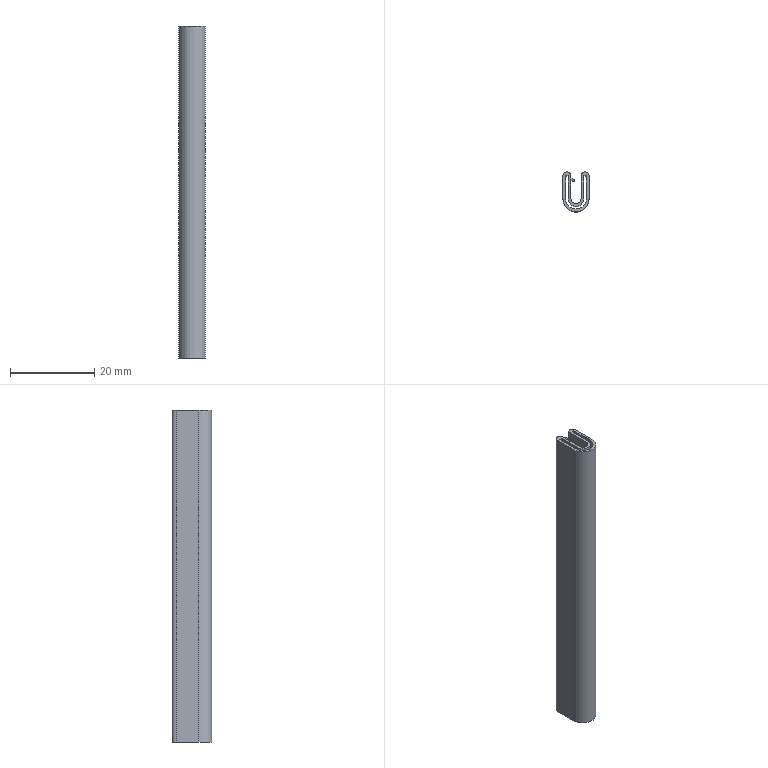Part | STEP file | TRAT2_4_B_3L2_TRAT2.4-B-3-L1 | 1 solid | 22 faces | box 6.2 x 9.5 x 79 mm | volume 2037 mm3 | plane 15 | cylinder 7 | commonest cylinder face diameters 1.9 x2 0.4 x1 2.4 x1 3.692 x1 4.933 x1 6.2 x1
STEP:
#1=CARTESIAN_POINT('',(1.9,8.55,79.));
#2=VERTEX_POINT('',#1);
#3=CARTESIAN_POINT('',(0.,8.55,79.));
#4=VERTEX_POINT('',#3);
#5=CARTESIAN_POINT('',(0.95,8.55,79.));
#6=DIRECTION('',(0.,0.,1.));
#7=DIRECTION('',(1.,0.,0.));
#8=AXIS2_PLACEMENT_3D('',#5,#6,#7);
#9=CIRCLE('',#8,0.95);
#10=EDGE_CURVE('',#2,#4,#9,.T.);
#11=ORIENTED_EDGE('',*,*,#10,.T.);
#12=CARTESIAN_POINT('',(0.,3.1,79.));
#13=VERTEX_POINT('',#12);
#14=CARTESIAN_POINT('',(0.,8.55,79.));
#15=DIRECTION('',(0.,-1.,0.));
#16=VECTOR('',#15,1000.);
#17=LINE('',#14,#16);
#18=EDGE_CURVE('',#4,#13,#17,.T.);
#19=ORIENTED_EDGE('',*,*,#18,.T.);
#20=CARTESIAN_POINT('',(6.2,3.1,79.));
#21=VERTEX_POINT('',#20);
#22=CARTESIAN_POINT('',(3.1,3.1,79.));
#23=DIRECTION('',(0.,0.,1.));
#24=DIRECTION('',(1.,0.,0.));
#25=AXIS2_PLACEMENT_3D('',#22,#23,#24);
#26=CIRCLE('',#25,3.1);
#27=EDGE_CURVE('',#13,#21,#26,.T.);
#28=ORIENTED_EDGE('',*,*,#27,.T.);
#29=CARTESIAN_POINT('',(6.2,8.55,79.));
#30=VERTEX_POINT('',#29);
#31=CARTESIAN_POINT('',(6.2,3.1,79.));
#32=DIRECTION('',(0.,1.,0.));
#33=VECTOR('',#32,1000.);
#34=LINE('',#31,#33);
#35=EDGE_CURVE('',#21,#30,#34,.T.);
#36=ORIENTED_EDGE('',*,*,#35,.T.);
#37=CARTESIAN_POINT('',(4.3,8.55,79.));
#38=VERTEX_POINT('',#37);
#39=CARTESIAN_POINT('',(5.25,8.55,79.));
#40=DIRECTION('',(0.,0.,1.));
#41=DIRECTION('',(1.,0.,0.));
#42=AXIS2_PLACEMENT_3D('',#39,#40,#41);
#43=CIRCLE('',#42,0.95);
#44=EDGE_CURVE('',#30,#38,#43,.T.);
#45=ORIENTED_EDGE('',*,*,#44,.T.);
#46=CARTESIAN_POINT('',(4.3,3.1,79.));
#47=VERTEX_POINT('',#46);
#48=CARTESIAN_POINT('',(4.3,8.55,79.));
#49=DIRECTION('',(0.,-1.,0.));
#50=VECTOR('',#49,1000.);
#51=LINE('',#48,#50);
#52=EDGE_CURVE('',#38,#47,#51,.T.);
#53=ORIENTED_EDGE('',*,*,#52,.T.);
#54=CARTESIAN_POINT('',(1.9,3.1,79.));
#55=VERTEX_POINT('',#54);
#56=CARTESIAN_POINT('',(3.1,3.1,79.));
#57=DIRECTION('',(0.,0.,-1.));
#58=DIRECTION('',(-1.,0.,0.));
#59=AXIS2_PLACEMENT_3D('',#56,#57,#58);
#60=CIRCLE('',#59,1.2);
#61=EDGE_CURVE('',#47,#55,#60,.T.);
#62=ORIENTED_EDGE('',*,*,#61,.T.);
#63=CARTESIAN_POINT('',(1.9,7.6,79.));
#64=VERTEX_POINT('',#63);
#65=CARTESIAN_POINT('',(1.9,3.1,79.));
#66=DIRECTION('',(0.,1.,0.));
#67=VECTOR('',#66,1000.);
#68=LINE('',#65,#67);
#69=EDGE_CURVE('',#55,#64,#68,.T.);
#70=ORIENTED_EDGE('',*,*,#69,.T.);
#71=CARTESIAN_POINT('',(2.472,7.27,79.));
#72=VERTEX_POINT('',#71);
#73=CARTESIAN_POINT('',(1.9,7.6,79.));
#74=DIRECTION('',(0.866,-0.5,0.));
#75=VECTOR('',#74,1000.);
#76=LINE('',#73,#75);
#77=EDGE_CURVE('',#64,#72,#76,.T.);
#78=ORIENTED_EDGE('',*,*,#77,.T.);
#79=CARTESIAN_POINT('',(2.672,7.616,79.));
#80=VERTEX_POINT('',#79);
#81=CARTESIAN_POINT('',(2.572,7.443,79.));
#82=DIRECTION('',(0.,0.,1.));
#83=DIRECTION('',(1.,0.,0.));
#84=AXIS2_PLACEMENT_3D('',#81,#82,#83);
#85=CIRCLE('',#84,0.2);
#86=EDGE_CURVE('',#72,#80,#85,.T.);
#87=ORIENTED_EDGE('',*,*,#86,.T.);
#88=CARTESIAN_POINT('',(1.9,8.062,79.));
#89=VERTEX_POINT('',#88);
#90=CARTESIAN_POINT('',(2.672,7.616,79.));
#91=DIRECTION('',(-0.866,0.5,0.));
#92=VECTOR('',#91,1000.);
#93=LINE('',#90,#92);
#94=EDGE_CURVE('',#80,#89,#93,.T.);
#95=ORIENTED_EDGE('',*,*,#94,.T.);
#96=CARTESIAN_POINT('',(1.9,8.062,79.));
#97=DIRECTION('',(0.,1.,0.));
#98=VECTOR('',#97,1000.);
#99=LINE('',#96,#98);
#100=EDGE_CURVE('',#89,#2,#99,.T.);
#101=ORIENTED_EDGE('',*,*,#100,.T.);
#102=EDGE_LOOP('',(#11,#19,#28,#36,#45,#53,#62,#70,#78,#87,#95,#101));
#103=FACE_OUTER_BOUND('',#102,.T.);
#104=CARTESIAN_POINT('',(0.6333,8.55,79.));
#105=VERTEX_POINT('',#104);
#106=CARTESIAN_POINT('',(0.6333,3.1,79.));
#107=VERTEX_POINT('',#106);
#108=CARTESIAN_POINT('',(0.6333,8.55,79.));
#109=DIRECTION('',(0.,-1.,0.));
#110=VECTOR('',#109,1000.);
#111=LINE('',#108,#110);
#112=EDGE_CURVE('',#105,#107,#111,.T.);
#113=ORIENTED_EDGE('',*,*,#112,.F.);
#114=CARTESIAN_POINT('',(1.254,8.55,79.));
#115=VERTEX_POINT('',#114);
#116=CARTESIAN_POINT('',(1.254,8.55,79.));
#117=DIRECTION('',(-1.,0.,0.));
#118=VECTOR('',#117,1000.);
#119=LINE('',#116,#118);
#120=EDGE_CURVE('',#115,#105,#119,.T.);
#121=ORIENTED_EDGE('',*,*,#120,.F.);
#122=CARTESIAN_POINT('',(1.254,3.1,79.));
#123=VERTEX_POINT('',#122);
#124=CARTESIAN_POINT('',(1.254,3.1,79.));
#125=DIRECTION('',(0.,1.,0.));
#126=VECTOR('',#125,1000.);
#127=LINE('',#124,#126);
#128=EDGE_CURVE('',#123,#115,#127,.T.);
#129=ORIENTED_EDGE('',*,*,#128,.F.);
#130=CARTESIAN_POINT('',(4.946,3.1,79.));
#131=VERTEX_POINT('',#130);
#132=CARTESIAN_POINT('',(3.1,3.1,79.));
#133=DIRECTION('',(0.,0.,-1.));
#134=DIRECTION('',(-1.,0.,0.));
#135=AXIS2_PLACEMENT_3D('',#132,#133,#134);
#136=CIRCLE('',#135,1.846);
#137=EDGE_CURVE('',#131,#123,#136,.T.);
#138=ORIENTED_EDGE('',*,*,#137,.F.);
#139=CARTESIAN_POINT('',(4.946,8.55,79.));
#140=VERTEX_POINT('',#139);
#141=CARTESIAN_POINT('',(4.946,8.55,79.));
#142=DIRECTION('',(0.,-1.,0.));
#143=VECTOR('',#142,1000.);
#144=LINE('',#141,#143);
#145=EDGE_CURVE('',#140,#131,#144,.T.);
#146=ORIENTED_EDGE('',*,*,#145,.F.);
#147=CARTESIAN_POINT('',(5.567,8.55,79.));
#148=VERTEX_POINT('',#147);
#149=CARTESIAN_POINT('',(5.567,8.55,79.));
#150=DIRECTION('',(-1.,0.,0.));
#151=VECTOR('',#150,1000.);
#152=LINE('',#149,#151);
#153=EDGE_CURVE('',#148,#140,#152,.T.);
#154=ORIENTED_EDGE('',*,*,#153,.F.);
#155=CARTESIAN_POINT('',(5.567,3.1,79.));
#156=VERTEX_POINT('',#155);
#157=CARTESIAN_POINT('',(5.567,3.1,79.));
#158=DIRECTION('',(0.,1.,0.));
#159=VECTOR('',#158,1000.);
#160=LINE('',#157,#159);
#161=EDGE_CURVE('',#156,#148,#160,.T.);
#162=ORIENTED_EDGE('',*,*,#161,.F.);
#163=CARTESIAN_POINT('',(3.1,3.1,79.));
#164=DIRECTION('',(0.,0.,1.));
#165=DIRECTION('',(1.,0.,0.));
#166=AXIS2_PLACEMENT_3D('',#163,#164,#165);
#167=CIRCLE('',#166,2.467);
#168=EDGE_CURVE('',#107,#156,#167,.T.);
#169=ORIENTED_EDGE('',*,*,#168,.F.);
#170=EDGE_LOOP('',(#113,#121,#129,#138,#146,#154,#162,#169));
#171=FACE_BOUND('',#170,.T.);
#172=CARTESIAN_POINT('',(0.95,8.55,79.));
#173=DIRECTION('',(0.,0.,1.));
#174=DIRECTION('',(1.,0.,0.));
#175=AXIS2_PLACEMENT_3D('',#172,#173,#174);
#176=PLANE('',#175);
#177=ADVANCED_FACE('',(#103,#171),#176,.T.);
#178=CARTESIAN_POINT('',(1.9,8.55,0.));
#179=VERTEX_POINT('',#178);
#180=CARTESIAN_POINT('',(0.,8.55,0.));
#181=VERTEX_POINT('',#180);
#182=CARTESIAN_POINT('',(0.95,8.55,0.));
#183=DIRECTION('',(0.,0.,1.));
#184=DIRECTION('',(1.,0.,0.));
#185=AXIS2_PLACEMENT_3D('',#182,#183,#184);
#186=CIRCLE('',#185,0.95);
#187=EDGE_CURVE('',#179,#181,#186,.T.);
#188=ORIENTED_EDGE('',*,*,#187,.F.);
#189=CARTESIAN_POINT('',(1.9,8.062,0.));
#190=VERTEX_POINT('',#189);
#191=CARTESIAN_POINT('',(1.9,8.062,0.));
#192=DIRECTION('',(0.,1.,0.));
#193=VECTOR('',#192,1000.);
#194=LINE('',#191,#193);
#195=EDGE_CURVE('',#190,#179,#194,.T.);
#196=ORIENTED_EDGE('',*,*,#195,.F.);
#197=CARTESIAN_POINT('',(2.672,7.616,0.));
#198=VERTEX_POINT('',#197);
#199=CARTESIAN_POINT('',(2.672,7.616,0.));
#200=DIRECTION('',(-0.866,0.5,0.));
#201=VECTOR('',#200,1000.);
#202=LINE('',#199,#201);
#203=EDGE_CURVE('',#198,#190,#202,.T.);
#204=ORIENTED_EDGE('',*,*,#203,.F.);
#205=CARTESIAN_POINT('',(2.472,7.27,0.));
#206=VERTEX_POINT('',#205);
#207=CARTESIAN_POINT('',(2.572,7.443,0.));
#208=DIRECTION('',(0.,0.,1.));
#209=DIRECTION('',(1.,0.,0.));
#210=AXIS2_PLACEMENT_3D('',#207,#208,#209);
#211=CIRCLE('',#210,0.2);
#212=EDGE_CURVE('',#206,#198,#211,.T.);
#213=ORIENTED_EDGE('',*,*,#212,.F.);
#214=CARTESIAN_POINT('',(1.9,7.6,0.));
#215=VERTEX_POINT('',#214);
#216=CARTESIAN_POINT('',(1.9,7.6,0.));
#217=DIRECTION('',(0.866,-0.5,0.));
#218=VECTOR('',#217,1000.);
#219=LINE('',#216,#218);
#220=EDGE_CURVE('',#215,#206,#219,.T.);
#221=ORIENTED_EDGE('',*,*,#220,.F.);
#222=CARTESIAN_POINT('',(1.9,3.1,0.));
#223=VERTEX_POINT('',#222);
#224=CARTESIAN_POINT('',(1.9,3.1,0.));
#225=DIRECTION('',(0.,1.,0.));
#226=VECTOR('',#225,1000.);
#227=LINE('',#224,#226);
#228=EDGE_CURVE('',#223,#215,#227,.T.);
#229=ORIENTED_EDGE('',*,*,#228,.F.);
#230=CARTESIAN_POINT('',(4.3,3.1,0.));
#231=VERTEX_POINT('',#230);
#232=CARTESIAN_POINT('',(3.1,3.1,0.));
#233=DIRECTION('',(0.,0.,-1.));
#234=DIRECTION('',(-1.,0.,0.));
#235=AXIS2_PLACEMENT_3D('',#232,#233,#234);
#236=CIRCLE('',#235,1.2);
#237=EDGE_CURVE('',#231,#223,#236,.T.);
#238=ORIENTED_EDGE('',*,*,#237,.F.);
#239=CARTESIAN_POINT('',(4.3,8.55,0.));
#240=VERTEX_POINT('',#239);
#241=CARTESIAN_POINT('',(4.3,8.55,0.));
#242=DIRECTION('',(0.,-1.,0.));
#243=VECTOR('',#242,1000.);
#244=LINE('',#241,#243);
#245=EDGE_CURVE('',#240,#231,#244,.T.);
#246=ORIENTED_EDGE('',*,*,#245,.F.);
#247=CARTESIAN_POINT('',(6.2,8.55,0.));
#248=VERTEX_POINT('',#247);
#249=CARTESIAN_POINT('',(5.25,8.55,0.));
#250=DIRECTION('',(0.,0.,1.));
#251=DIRECTION('',(1.,0.,0.));
#252=AXIS2_PLACEMENT_3D('',#249,#250,#251);
#253=CIRCLE('',#252,0.95);
#254=EDGE_CURVE('',#248,#240,#253,.T.);
#255=ORIENTED_EDGE('',*,*,#254,.F.);
#256=CARTESIAN_POINT('',(6.2,3.1,0.));
#257=VERTEX_POINT('',#256);
#258=CARTESIAN_POINT('',(6.2,3.1,0.));
#259=DIRECTION('',(0.,1.,0.));
#260=VECTOR('',#259,1000.);
#261=LINE('',#258,#260);
#262=EDGE_CURVE('',#257,#248,#261,.T.);
#263=ORIENTED_EDGE('',*,*,#262,.F.);
#264=CARTESIAN_POINT('',(0.,3.1,0.));
#265=VERTEX_POINT('',#264);
#266=CARTESIAN_POINT('',(3.1,3.1,0.));
#267=DIRECTION('',(0.,0.,1.));
#268=DIRECTION('',(1.,0.,0.));
#269=AXIS2_PLACEMENT_3D('',#266,#267,#268);
#270=CIRCLE('',#269,3.1);
#271=EDGE_CURVE('',#265,#257,#270,.T.);
#272=ORIENTED_EDGE('',*,*,#271,.F.);
#273=CARTESIAN_POINT('',(0.,8.55,0.));
#274=DIRECTION('',(0.,-1.,0.));
#275=VECTOR('',#274,1000.);
#276=LINE('',#273,#275);
#277=EDGE_CURVE('',#181,#265,#276,.T.);
#278=ORIENTED_EDGE('',*,*,#277,.F.);
#279=EDGE_LOOP('',(#188,#196,#204,#213,#221,#229,#238,#246,#255,#263,#272,#278));
#280=FACE_OUTER_BOUND('',#279,.T.);
#281=CARTESIAN_POINT('',(1.254,8.55,0.));
#282=VERTEX_POINT('',#281);
#283=CARTESIAN_POINT('',(0.6333,8.55,0.));
#284=VERTEX_POINT('',#283);
#285=CARTESIAN_POINT('',(1.254,8.55,0.));
#286=DIRECTION('',(-1.,0.,0.));
#287=VECTOR('',#286,1000.);
#288=LINE('',#285,#287);
#289=EDGE_CURVE('',#282,#284,#288,.T.);
#290=ORIENTED_EDGE('',*,*,#289,.T.);
#291=CARTESIAN_POINT('',(0.6333,3.1,0.));
#292=VERTEX_POINT('',#291);
#293=CARTESIAN_POINT('',(0.6333,8.55,0.));
#294=DIRECTION('',(0.,-1.,0.));
#295=VECTOR('',#294,1000.);
#296=LINE('',#293,#295);
#297=EDGE_CURVE('',#284,#292,#296,.T.);
#298=ORIENTED_EDGE('',*,*,#297,.T.);
#299=CARTESIAN_POINT('',(5.567,3.1,0.));
#300=VERTEX_POINT('',#299);
#301=CARTESIAN_POINT('',(3.1,3.1,0.));
#302=DIRECTION('',(0.,0.,1.));
#303=DIRECTION('',(1.,0.,0.));
#304=AXIS2_PLACEMENT_3D('',#301,#302,#303);
#305=CIRCLE('',#304,2.467);
#306=EDGE_CURVE('',#292,#300,#305,.T.);
#307=ORIENTED_EDGE('',*,*,#306,.T.);
#308=CARTESIAN_POINT('',(5.567,8.55,0.));
#309=VERTEX_POINT('',#308);
#310=CARTESIAN_POINT('',(5.567,3.1,0.));
#311=DIRECTION('',(0.,1.,0.));
#312=VECTOR('',#311,1000.);
#313=LINE('',#310,#312);
#314=EDGE_CURVE('',#300,#309,#313,.T.);
#315=ORIENTED_EDGE('',*,*,#314,.T.);
#316=CARTESIAN_POINT('',(4.946,8.55,0.));
#317=VERTEX_POINT('',#316);
#318=CARTESIAN_POINT('',(5.567,8.55,0.));
#319=DIRECTION('',(-1.,0.,0.));
#320=VECTOR('',#319,1000.);
#321=LINE('',#318,#320);
#322=EDGE_CURVE('',#309,#317,#321,.T.);
#323=ORIENTED_EDGE('',*,*,#322,.T.);
#324=CARTESIAN_POINT('',(4.946,3.1,0.));
#325=VERTEX_POINT('',#324);
#326=CARTESIAN_POINT('',(4.946,8.55,0.));
#327=DIRECTION('',(0.,-1.,0.));
#328=VECTOR('',#327,1000.);
#329=LINE('',#326,#328);
#330=EDGE_CURVE('',#317,#325,#329,.T.);
#331=ORIENTED_EDGE('',*,*,#330,.T.);
#332=CARTESIAN_POINT('',(1.254,3.1,0.));
#333=VERTEX_POINT('',#332);
#334=CARTESIAN_POINT('',(3.1,3.1,0.));
#335=DIRECTION('',(0.,0.,-1.));
#336=DIRECTION('',(-1.,0.,0.));
#337=AXIS2_PLACEMENT_3D('',#334,#335,#336);
#338=CIRCLE('',#337,1.846);
#339=EDGE_CURVE('',#325,#333,#338,.T.);
#340=ORIENTED_EDGE('',*,*,#339,.T.);
#341=CARTESIAN_POINT('',(1.254,3.1,0.));
#342=DIRECTION('',(0.,1.,0.));
#343=VECTOR('',#342,1000.);
#344=LINE('',#341,#343);
#345=EDGE_CURVE('',#333,#282,#344,.T.);
#346=ORIENTED_EDGE('',*,*,#345,.T.);
#347=EDGE_LOOP('',(#290,#298,#307,#315,#323,#331,#340,#346));
#348=FACE_BOUND('',#347,.T.);
#349=CARTESIAN_POINT('',(0.95,8.55,0.));
#350=DIRECTION('',(0.,0.,1.));
#351=DIRECTION('',(1.,0.,0.));
#352=AXIS2_PLACEMENT_3D('',#349,#350,#351);
#353=PLANE('',#352);
#354=ADVANCED_FACE('',(#280,#348),#353,.F.);
#355=ORIENTED_EDGE('',*,*,#187,.T.);
#356=CARTESIAN_POINT('',(0.,8.55,79.));
#357=DIRECTION('',(0.,0.,-1.));
#358=VECTOR('',#357,1000.);
#359=LINE('',#356,#358);
#360=EDGE_CURVE('',#4,#181,#359,.T.);
#361=ORIENTED_EDGE('',*,*,#360,.F.);
#362=ORIENTED_EDGE('',*,*,#10,.F.);
#363=CARTESIAN_POINT('',(1.9,8.55,79.));
#364=DIRECTION('',(0.,0.,-1.));
#365=VECTOR('',#364,1000.);
#366=LINE('',#363,#365);
#367=EDGE_CURVE('',#2,#179,#366,.T.);
#368=ORIENTED_EDGE('',*,*,#367,.T.);
#369=EDGE_LOOP('',(#355,#361,#362,#368));
#370=FACE_OUTER_BOUND('',#369,.T.);
#371=CARTESIAN_POINT('',(0.95,8.55,79.));
#372=DIRECTION('',(0.,0.,-1.));
#373=DIRECTION('',(-1.,0.,0.));
#374=AXIS2_PLACEMENT_3D('',#371,#372,#373);
#375=CYLINDRICAL_SURFACE('',#374,0.95);
#376=ADVANCED_FACE('',(#370),#375,.T.);
#377=ORIENTED_EDGE('',*,*,#277,.T.);
#378=CARTESIAN_POINT('',(0.,3.1,79.));
#379=DIRECTION('',(0.,0.,-1.));
#380=VECTOR('',#379,1000.);
#381=LINE('',#378,#380);
#382=EDGE_CURVE('',#13,#265,#381,.T.);
#383=ORIENTED_EDGE('',*,*,#382,.F.);
#384=ORIENTED_EDGE('',*,*,#18,.F.);
#385=ORIENTED_EDGE('',*,*,#360,.T.);
#386=EDGE_LOOP('',(#377,#383,#384,#385));
#387=FACE_OUTER_BOUND('',#386,.T.);
#388=CARTESIAN_POINT('',(0.,8.55,79.));
#389=DIRECTION('',(1.,0.,0.));
#390=DIRECTION('',(0.,0.,-1.));
#391=AXIS2_PLACEMENT_3D('',#388,#389,#390);
#392=PLANE('',#391);
#393=ADVANCED_FACE('',(#387),#392,.F.);
#394=ORIENTED_EDGE('',*,*,#271,.T.);
#395=CARTESIAN_POINT('',(6.2,3.1,79.));
#396=DIRECTION('',(0.,0.,-1.));
#397=VECTOR('',#396,1000.);
#398=LINE('',#395,#397);
#399=EDGE_CURVE('',#21,#257,#398,.T.);
#400=ORIENTED_EDGE('',*,*,#399,.F.);
#401=ORIENTED_EDGE('',*,*,#27,.F.);
#402=ORIENTED_EDGE('',*,*,#382,.T.);
#403=EDGE_LOOP('',(#394,#400,#401,#402));
#404=FACE_OUTER_BOUND('',#403,.T.);
#405=CARTESIAN_POINT('',(3.1,3.1,79.));
#406=DIRECTION('',(0.,0.,-1.));
#407=DIRECTION('',(-1.,0.,0.));
#408=AXIS2_PLACEMENT_3D('',#405,#406,#407);
#409=CYLINDRICAL_SURFACE('',#408,3.1);
#410=ADVANCED_FACE('',(#404),#409,.T.);
#411=ORIENTED_EDGE('',*,*,#262,.T.);
#412=CARTESIAN_POINT('',(6.2,8.55,79.));
#413=DIRECTION('',(0.,0.,-1.));
#414=VECTOR('',#413,1000.);
#415=LINE('',#412,#414);
#416=EDGE_CURVE('',#30,#248,#415,.T.);
#417=ORIENTED_EDGE('',*,*,#416,.F.);
#418=ORIENTED_EDGE('',*,*,#35,.F.);
#419=ORIENTED_EDGE('',*,*,#399,.T.);
#420=EDGE_LOOP('',(#411,#417,#418,#419));
#421=FACE_OUTER_BOUND('',#420,.T.);
#422=CARTESIAN_POINT('',(6.2,3.1,79.));
#423=DIRECTION('',(-1.,0.,0.));
#424=DIRECTION('',(0.,0.,1.));
#425=AXIS2_PLACEMENT_3D('',#422,#423,#424);
#426=PLANE('',#425);
#427=ADVANCED_FACE('',(#421),#426,.F.);
#428=ORIENTED_EDGE('',*,*,#254,.T.);
#429=CARTESIAN_POINT('',(4.3,8.55,79.));
#430=DIRECTION('',(0.,0.,-1.));
#431=VECTOR('',#430,1000.);
#432=LINE('',#429,#431);
#433=EDGE_CURVE('',#38,#240,#432,.T.);
#434=ORIENTED_EDGE('',*,*,#433,.F.);
#435=ORIENTED_EDGE('',*,*,#44,.F.);
#436=ORIENTED_EDGE('',*,*,#416,.T.);
#437=EDGE_LOOP('',(#428,#434,#435,#436));
#438=FACE_OUTER_BOUND('',#437,.T.);
#439=CARTESIAN_POINT('',(5.25,8.55,79.));
#440=DIRECTION('',(0.,0.,-1.));
#441=DIRECTION('',(-1.,0.,0.));
#442=AXIS2_PLACEMENT_3D('',#439,#440,#441);
#443=CYLINDRICAL_SURFACE('',#442,0.95);
#444=ADVANCED_FACE('',(#438),#443,.T.);
#445=ORIENTED_EDGE('',*,*,#245,.T.);
#446=CARTESIAN_POINT('',(4.3,3.1,79.));
#447=DIRECTION('',(0.,0.,-1.));
#448=VECTOR('',#447,1000.);
#449=LINE('',#446,#448);
#450=EDGE_CURVE('',#47,#231,#449,.T.);
#451=ORIENTED_EDGE('',*,*,#450,.F.);
#452=ORIENTED_EDGE('',*,*,#52,.F.);
#453=ORIENTED_EDGE('',*,*,#433,.T.);
#454=EDGE_LOOP('',(#445,#451,#452,#453));
#455=FACE_OUTER_BOUND('',#454,.T.);
#456=CARTESIAN_POINT('',(4.3,8.55,79.));
#457=DIRECTION('',(1.,0.,0.));
#458=DIRECTION('',(0.,1.,0.));
#459=AXIS2_PLACEMENT_3D('',#456,#457,#458);
#460=PLANE('',#459);
#461=ADVANCED_FACE('',(#455),#460,.F.);
#462=ORIENTED_EDGE('',*,*,#237,.T.);
#463=CARTESIAN_POINT('',(1.9,3.1,79.));
#464=DIRECTION('',(0.,0.,-1.));
#465=VECTOR('',#464,1000.);
#466=LINE('',#463,#465);
#467=EDGE_CURVE('',#55,#223,#466,.T.);
#468=ORIENTED_EDGE('',*,*,#467,.F.);
#469=ORIENTED_EDGE('',*,*,#61,.F.);
#470=ORIENTED_EDGE('',*,*,#450,.T.);
#471=EDGE_LOOP('',(#462,#468,#469,#470));
#472=FACE_OUTER_BOUND('',#471,.T.);
#473=CARTESIAN_POINT('',(3.1,3.1,79.));
#474=DIRECTION('',(0.,0.,-1.));
#475=DIRECTION('',(-1.,0.,0.));
#476=AXIS2_PLACEMENT_3D('',#473,#474,#475);
#477=CYLINDRICAL_SURFACE('',#476,1.2);
#478=ADVANCED_FACE('',(#472),#477,.F.);
#479=ORIENTED_EDGE('',*,*,#228,.T.);
#480=CARTESIAN_POINT('',(1.9,7.6,79.));
#481=DIRECTION('',(0.,0.,-1.));
#482=VECTOR('',#481,1000.);
#483=LINE('',#480,#482);
#484=EDGE_CURVE('',#64,#215,#483,.T.);
#485=ORIENTED_EDGE('',*,*,#484,.F.);
#486=ORIENTED_EDGE('',*,*,#69,.F.);
#487=ORIENTED_EDGE('',*,*,#467,.T.);
#488=EDGE_LOOP('',(#479,#485,#486,#487));
#489=FACE_OUTER_BOUND('',#488,.T.);
#490=CARTESIAN_POINT('',(1.9,3.1,79.));
#491=DIRECTION('',(-1.,0.,0.));
#492=DIRECTION('',(0.,-1.,0.));
#493=AXIS2_PLACEMENT_3D('',#490,#491,#492);
#494=PLANE('',#493);
#495=ADVANCED_FACE('',(#489),#494,.F.);
#496=ORIENTED_EDGE('',*,*,#220,.T.);
#497=CARTESIAN_POINT('',(2.472,7.27,79.));
#498=DIRECTION('',(0.,0.,-1.));
#499=VECTOR('',#498,1000.);
#500=LINE('',#497,#499);
#501=EDGE_CURVE('',#72,#206,#500,.T.);
#502=ORIENTED_EDGE('',*,*,#501,.F.);
#503=ORIENTED_EDGE('',*,*,#77,.F.);
#504=ORIENTED_EDGE('',*,*,#484,.T.);
#505=EDGE_LOOP('',(#496,#502,#503,#504));
#506=FACE_OUTER_BOUND('',#505,.T.);
#507=CARTESIAN_POINT('',(1.9,7.6,79.));
#508=DIRECTION('',(0.5,0.866,0.));
#509=DIRECTION('',(-0.866,0.5,0.));
#510=AXIS2_PLACEMENT_3D('',#507,#508,#509);
#511=PLANE('',#510);
#512=ADVANCED_FACE('',(#506),#511,.F.);
#513=ORIENTED_EDGE('',*,*,#212,.T.);
#514=CARTESIAN_POINT('',(2.672,7.616,79.));
#515=DIRECTION('',(0.,0.,-1.));
#516=VECTOR('',#515,1000.);
#517=LINE('',#514,#516);
#518=EDGE_CURVE('',#80,#198,#517,.T.);
#519=ORIENTED_EDGE('',*,*,#518,.F.);
#520=ORIENTED_EDGE('',*,*,#86,.F.);
#521=ORIENTED_EDGE('',*,*,#501,.T.);
#522=EDGE_LOOP('',(#513,#519,#520,#521));
#523=FACE_OUTER_BOUND('',#522,.T.);
#524=CARTESIAN_POINT('',(2.572,7.443,79.));
#525=DIRECTION('',(0.,0.,-1.));
#526=DIRECTION('',(-1.,0.,0.));
#527=AXIS2_PLACEMENT_3D('',#524,#525,#526);
#528=CYLINDRICAL_SURFACE('',#527,0.2);
#529=ADVANCED_FACE('',(#523),#528,.T.);
#530=ORIENTED_EDGE('',*,*,#203,.T.);
#531=CARTESIAN_POINT('',(1.9,8.062,79.));
#532=DIRECTION('',(0.,0.,-1.));
#533=VECTOR('',#532,1000.);
#534=LINE('',#531,#533);
#535=EDGE_CURVE('',#89,#190,#534,.T.);
#536=ORIENTED_EDGE('',*,*,#535,.F.);
#537=ORIENTED_EDGE('',*,*,#94,.F.);
#538=ORIENTED_EDGE('',*,*,#518,.T.);
#539=EDGE_LOOP('',(#530,#536,#537,#538));
#540=FACE_OUTER_BOUND('',#539,.T.);
#541=CARTESIAN_POINT('',(2.672,7.616,79.));
#542=DIRECTION('',(-0.5,-0.866,0.));
#543=DIRECTION('',(0.866,-0.5,0.));
#544=AXIS2_PLACEMENT_3D('',#541,#542,#543);
#545=PLANE('',#544);
#546=ADVANCED_FACE('',(#540),#545,.F.);
#547=ORIENTED_EDGE('',*,*,#195,.T.);
#548=ORIENTED_EDGE('',*,*,#367,.F.);
#549=ORIENTED_EDGE('',*,*,#100,.F.);
#550=ORIENTED_EDGE('',*,*,#535,.T.);
#551=EDGE_LOOP('',(#547,#548,#549,#550));
#552=FACE_OUTER_BOUND('',#551,.T.);
#553=CARTESIAN_POINT('',(1.9,8.062,79.));
#554=DIRECTION('',(-1.,0.,0.));
#555=DIRECTION('',(0.,0.,1.));
#556=AXIS2_PLACEMENT_3D('',#553,#554,#555);
#557=PLANE('',#556);
#558=ADVANCED_FACE('',(#552),#557,.F.);
#559=ORIENTED_EDGE('',*,*,#289,.F.);
#560=CARTESIAN_POINT('',(1.254,8.55,79.));
#561=DIRECTION('',(0.,0.,-1.));
#562=VECTOR('',#561,1000.);
#563=LINE('',#560,#562);
#564=EDGE_CURVE('',#115,#282,#563,.T.);
#565=ORIENTED_EDGE('',*,*,#564,.F.);
#566=ORIENTED_EDGE('',*,*,#120,.T.);
#567=CARTESIAN_POINT('',(0.6333,8.55,79.));
#568=DIRECTION('',(0.,0.,-1.));
#569=VECTOR('',#568,1000.);
#570=LINE('',#567,#569);
#571=EDGE_CURVE('',#105,#284,#570,.T.);
#572=ORIENTED_EDGE('',*,*,#571,.T.);
#573=EDGE_LOOP('',(#559,#565,#566,#572));
#574=FACE_OUTER_BOUND('',#573,.T.);
#575=CARTESIAN_POINT('',(1.254,8.55,79.));
#576=DIRECTION('',(0.,-1.,0.));
#577=DIRECTION('',(0.,0.,-1.));
#578=AXIS2_PLACEMENT_3D('',#575,#576,#577);
#579=PLANE('',#578);
#580=ADVANCED_FACE('',(#574),#579,.T.);
#581=ORIENTED_EDGE('',*,*,#297,.F.);
#582=ORIENTED_EDGE('',*,*,#571,.F.);
#583=ORIENTED_EDGE('',*,*,#112,.T.);
#584=CARTESIAN_POINT('',(0.6333,3.1,79.));
#585=DIRECTION('',(0.,0.,-1.));
#586=VECTOR('',#585,1000.);
#587=LINE('',#584,#586);
#588=EDGE_CURVE('',#107,#292,#587,.T.);
#589=ORIENTED_EDGE('',*,*,#588,.T.);
#590=EDGE_LOOP('',(#581,#582,#583,#589));
#591=FACE_OUTER_BOUND('',#590,.T.);
#592=CARTESIAN_POINT('',(0.6333,8.55,79.));
#593=DIRECTION('',(1.,0.,0.));
#594=DIRECTION('',(0.,1.,0.));
#595=AXIS2_PLACEMENT_3D('',#592,#593,#594);
#596=PLANE('',#595);
#597=ADVANCED_FACE('',(#591),#596,.T.);
#598=ORIENTED_EDGE('',*,*,#306,.F.);
#599=ORIENTED_EDGE('',*,*,#588,.F.);
#600=ORIENTED_EDGE('',*,*,#168,.T.);
#601=CARTESIAN_POINT('',(5.567,3.1,79.));
#602=DIRECTION('',(0.,0.,-1.));
#603=VECTOR('',#602,1000.);
#604=LINE('',#601,#603);
#605=EDGE_CURVE('',#156,#300,#604,.T.);
#606=ORIENTED_EDGE('',*,*,#605,.T.);
#607=EDGE_LOOP('',(#598,#599,#600,#606));
#608=FACE_OUTER_BOUND('',#607,.T.);
#609=CARTESIAN_POINT('',(3.1,3.1,79.));
#610=DIRECTION('',(0.,0.,-1.));
#611=DIRECTION('',(-1.,0.,0.));
#612=AXIS2_PLACEMENT_3D('',#609,#610,#611);
#613=CYLINDRICAL_SURFACE('',#612,2.467);
#614=ADVANCED_FACE('',(#608),#613,.F.);
#615=ORIENTED_EDGE('',*,*,#314,.F.);
#616=ORIENTED_EDGE('',*,*,#605,.F.);
#617=ORIENTED_EDGE('',*,*,#161,.T.);
#618=CARTESIAN_POINT('',(5.567,8.55,79.));
#619=DIRECTION('',(0.,0.,-1.));
#620=VECTOR('',#619,1000.);
#621=LINE('',#618,#620);
#622=EDGE_CURVE('',#148,#309,#621,.T.);
#623=ORIENTED_EDGE('',*,*,#622,.T.);
#624=EDGE_LOOP('',(#615,#616,#617,#623));
#625=FACE_OUTER_BOUND('',#624,.T.);
#626=CARTESIAN_POINT('',(5.567,3.1,79.));
#627=DIRECTION('',(-1.,0.,0.));
#628=DIRECTION('',(0.,-1.,0.));
#629=AXIS2_PLACEMENT_3D('',#626,#627,#628);
#630=PLANE('',#629);
#631=ADVANCED_FACE('',(#625),#630,.T.);
#632=ORIENTED_EDGE('',*,*,#322,.F.);
#633=ORIENTED_EDGE('',*,*,#622,.F.);
#634=ORIENTED_EDGE('',*,*,#153,.T.);
#635=CARTESIAN_POINT('',(4.946,8.55,79.));
#636=DIRECTION('',(0.,0.,-1.));
#637=VECTOR('',#636,1000.);
#638=LINE('',#635,#637);
#639=EDGE_CURVE('',#140,#317,#638,.T.);
#640=ORIENTED_EDGE('',*,*,#639,.T.);
#641=EDGE_LOOP('',(#632,#633,#634,#640));
#642=FACE_OUTER_BOUND('',#641,.T.);
#643=CARTESIAN_POINT('',(5.567,8.55,79.));
#644=DIRECTION('',(0.,-1.,0.));
#645=DIRECTION('',(0.,0.,-1.));
#646=AXIS2_PLACEMENT_3D('',#643,#644,#645);
#647=PLANE('',#646);
#648=ADVANCED_FACE('',(#642),#647,.T.);
#649=ORIENTED_EDGE('',*,*,#330,.F.);
#650=ORIENTED_EDGE('',*,*,#639,.F.);
#651=ORIENTED_EDGE('',*,*,#145,.T.);
#652=CARTESIAN_POINT('',(4.946,3.1,79.));
#653=DIRECTION('',(0.,0.,-1.));
#654=VECTOR('',#653,1000.);
#655=LINE('',#652,#654);
#656=EDGE_CURVE('',#131,#325,#655,.T.);
#657=ORIENTED_EDGE('',*,*,#656,.T.);
#658=EDGE_LOOP('',(#649,#650,#651,#657));
#659=FACE_OUTER_BOUND('',#658,.T.);
#660=CARTESIAN_POINT('',(4.946,8.55,79.));
#661=DIRECTION('',(1.,0.,0.));
#662=DIRECTION('',(0.,0.,-1.));
#663=AXIS2_PLACEMENT_3D('',#660,#661,#662);
#664=PLANE('',#663);
#665=ADVANCED_FACE('',(#659),#664,.T.);
#666=ORIENTED_EDGE('',*,*,#339,.F.);
#667=ORIENTED_EDGE('',*,*,#656,.F.);
#668=ORIENTED_EDGE('',*,*,#137,.T.);
#669=CARTESIAN_POINT('',(1.254,3.1,79.));
#670=DIRECTION('',(0.,0.,-1.));
#671=VECTOR('',#670,1000.);
#672=LINE('',#669,#671);
#673=EDGE_CURVE('',#123,#333,#672,.T.);
#674=ORIENTED_EDGE('',*,*,#673,.T.);
#675=EDGE_LOOP('',(#666,#667,#668,#674));
#676=FACE_OUTER_BOUND('',#675,.T.);
#677=CARTESIAN_POINT('',(3.1,3.1,79.));
#678=DIRECTION('',(0.,0.,-1.));
#679=DIRECTION('',(-1.,0.,0.));
#680=AXIS2_PLACEMENT_3D('',#677,#678,#679);
#681=CYLINDRICAL_SURFACE('',#680,1.846);
#682=ADVANCED_FACE('',(#676),#681,.T.);
#683=ORIENTED_EDGE('',*,*,#345,.F.);
#684=ORIENTED_EDGE('',*,*,#673,.F.);
#685=ORIENTED_EDGE('',*,*,#128,.T.);
#686=ORIENTED_EDGE('',*,*,#564,.T.);
#687=EDGE_LOOP('',(#683,#684,#685,#686));
#688=FACE_OUTER_BOUND('',#687,.T.);
#689=CARTESIAN_POINT('',(1.254,3.1,79.));
#690=DIRECTION('',(-1.,0.,0.));
#691=DIRECTION('',(0.,-1.,0.));
#692=AXIS2_PLACEMENT_3D('',#689,#690,#691);
#693=PLANE('',#692);
#694=ADVANCED_FACE('',(#688),#693,.T.);
#695=CLOSED_SHELL('',(#177,#354,#376,#393,#410,#427,#444,#461,#478,#495,#512,#529,#546,#558,#580,#597,#614,#631,#648,#665,#682,#694));
#696=MANIFOLD_SOLID_BREP('',#695);
#697=CARTESIAN_POINT('',(0.,0.,0.));
#698=DIRECTION('',(0.,0.,1.));
#699=DIRECTION('',(1.,0.,0.));
#700=AXIS2_PLACEMENT_3D('',#697,#698,#699);
#701=(LENGTH_UNIT()NAMED_UNIT(*)SI_UNIT(.MILLI.,.METRE.));
#702=UNCERTAINTY_MEASURE_WITH_UNIT(LENGTH_MEASURE(0.00001),#701,'','');
#703=(NAMED_UNIT(*)PLANE_ANGLE_UNIT()SI_UNIT($,.RADIAN.));
#704=(NAMED_UNIT(*)SI_UNIT($,.STERADIAN.)SOLID_ANGLE_UNIT());
#705=(GEOMETRIC_REPRESENTATION_CONTEXT(3)GLOBAL_UNCERTAINTY_ASSIGNED_CONTEXT((#702))GLOBAL_UNIT_ASSIGNED_CONTEXT((#701,#703,#704))REPRESENTATION_CONTEXT('',''));
#706=ADVANCED_BREP_SHAPE_REPRESENTATION('',(#696,#700),#705);